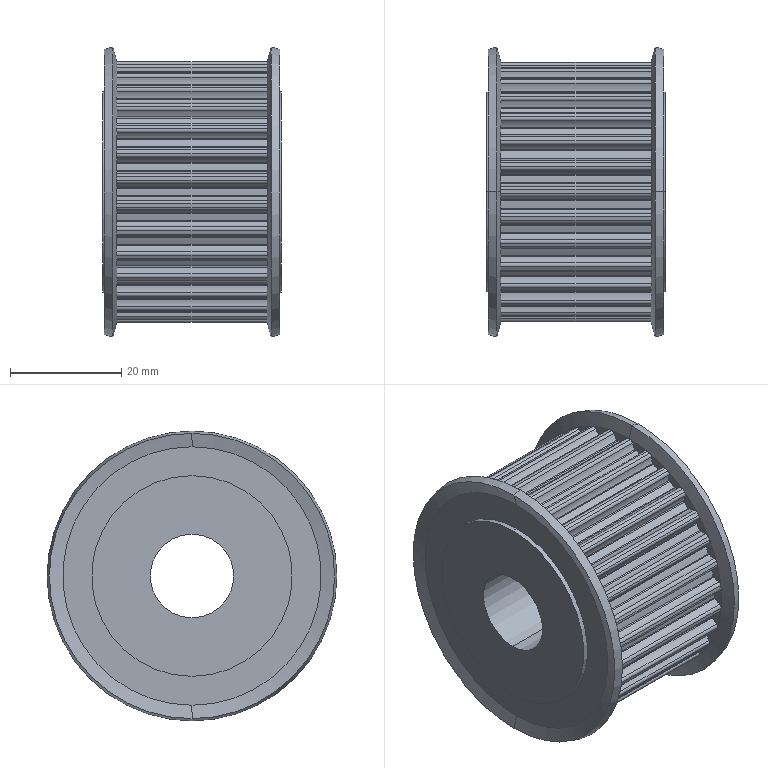Part | SolidWorks | 1 solid | 323 faces | box 32 x 52 x 52 mm | volume 45513 mm3 | cylinder 247 | plane 64 | cone 12 | commonest cylinder face diameters 0.5 x60 1.1 x60 6.55 x60 46.79 x31 43.25 x30 36 x4